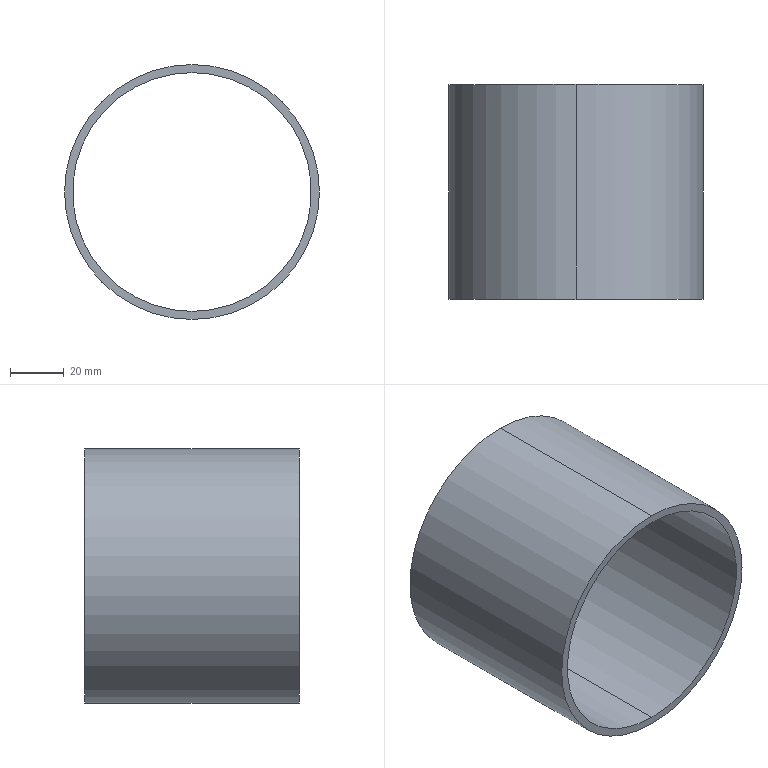Part | SolidWorks | features Extrusion 1 | 1 solid | 6 faces | box 95 x 80 x 95 mm | volume 69366 mm3 | cylinder 4 | plane 2 | commonest cylinder face diameters 89 x2 95 x2
STEP:
#1=CARTESIAN_POINT('',(0.,80.,-44.5));
#2=VERTEX_POINT('',#1);
#3=CARTESIAN_POINT('',(0.,80.,44.5));
#4=VERTEX_POINT('',#3);
#5=CARTESIAN_POINT('',(0.,80.,0.));
#6=DIRECTION('',(0.,1.,0.));
#7=DIRECTION('',(0.,0.,1.));
#8=AXIS2_PLACEMENT_3D('',#5,#6,#7);
#9=CIRCLE('',#8,44.5);
#10=EDGE_CURVE('',#2,#4,#9,.T.);
#11=ORIENTED_EDGE('',*,*,#10,.T.);
#12=CARTESIAN_POINT('',(0.,0.,44.5));
#13=VERTEX_POINT('',#12);
#14=CARTESIAN_POINT('',(0.,80.,44.5));
#15=DIRECTION('',(0.,-1.,0.));
#16=VECTOR('',#15,1000.);
#17=LINE('',#14,#16);
#18=EDGE_CURVE('',#4,#13,#17,.T.);
#19=ORIENTED_EDGE('',*,*,#18,.T.);
#20=CARTESIAN_POINT('',(0.,0.,-44.5));
#21=VERTEX_POINT('',#20);
#22=CARTESIAN_POINT('',(0.,0.,0.));
#23=DIRECTION('',(0.,1.,0.));
#24=DIRECTION('',(0.,0.,1.));
#25=AXIS2_PLACEMENT_3D('',#22,#23,#24);
#26=CIRCLE('',#25,44.5);
#27=EDGE_CURVE('',#21,#13,#26,.T.);
#28=ORIENTED_EDGE('',*,*,#27,.F.);
#29=CARTESIAN_POINT('',(0.,80.,-44.5));
#30=DIRECTION('',(0.,-1.,0.));
#31=VECTOR('',#30,1000.);
#32=LINE('',#29,#31);
#33=EDGE_CURVE('',#2,#21,#32,.T.);
#34=ORIENTED_EDGE('',*,*,#33,.F.);
#35=EDGE_LOOP('',(#11,#19,#28,#34));
#36=FACE_OUTER_BOUND('',#35,.T.);
#37=CARTESIAN_POINT('',(0.,80.,0.));
#38=DIRECTION('',(0.,-1.,0.));
#39=DIRECTION('',(0.,0.,-1.));
#40=AXIS2_PLACEMENT_3D('',#37,#38,#39);
#41=CYLINDRICAL_SURFACE('',#40,44.5);
#42=ADVANCED_FACE('',(#36),#41,.F.);
#43=CARTESIAN_POINT('',(0.,80.,47.5));
#44=VERTEX_POINT('',#43);
#45=CARTESIAN_POINT('',(0.,80.,-47.5));
#46=VERTEX_POINT('',#45);
#47=CARTESIAN_POINT('',(0.,80.,0.));
#48=DIRECTION('',(0.,1.,0.));
#49=DIRECTION('',(0.,0.,1.));
#50=AXIS2_PLACEMENT_3D('',#47,#48,#49);
#51=CIRCLE('',#50,47.5);
#52=EDGE_CURVE('',#44,#46,#51,.T.);
#53=ORIENTED_EDGE('',*,*,#52,.F.);
#54=CARTESIAN_POINT('',(0.,0.,47.5));
#55=VERTEX_POINT('',#54);
#56=CARTESIAN_POINT('',(0.,80.,47.5));
#57=DIRECTION('',(0.,-1.,0.));
#58=VECTOR('',#57,1000.);
#59=LINE('',#56,#58);
#60=EDGE_CURVE('',#44,#55,#59,.T.);
#61=ORIENTED_EDGE('',*,*,#60,.T.);
#62=CARTESIAN_POINT('',(0.,0.,-47.5));
#63=VERTEX_POINT('',#62);
#64=CARTESIAN_POINT('',(0.,0.,0.));
#65=DIRECTION('',(0.,1.,0.));
#66=DIRECTION('',(0.,0.,1.));
#67=AXIS2_PLACEMENT_3D('',#64,#65,#66);
#68=CIRCLE('',#67,47.5);
#69=EDGE_CURVE('',#55,#63,#68,.T.);
#70=ORIENTED_EDGE('',*,*,#69,.T.);
#71=CARTESIAN_POINT('',(0.,80.,-47.5));
#72=DIRECTION('',(0.,-1.,0.));
#73=VECTOR('',#72,1000.);
#74=LINE('',#71,#73);
#75=EDGE_CURVE('',#46,#63,#74,.T.);
#76=ORIENTED_EDGE('',*,*,#75,.F.);
#77=EDGE_LOOP('',(#53,#61,#70,#76));
#78=FACE_OUTER_BOUND('',#77,.T.);
#79=CARTESIAN_POINT('',(0.,80.,0.));
#80=DIRECTION('',(0.,-1.,0.));
#81=DIRECTION('',(0.,0.,-1.));
#82=AXIS2_PLACEMENT_3D('',#79,#80,#81);
#83=CYLINDRICAL_SURFACE('',#82,47.5);
#84=ADVANCED_FACE('',(#78),#83,.T.);
#85=CARTESIAN_POINT('',(0.,80.,0.));
#86=DIRECTION('',(0.,1.,0.));
#87=DIRECTION('',(0.,0.,1.));
#88=AXIS2_PLACEMENT_3D('',#85,#86,#87);
#89=CIRCLE('',#88,47.5);
#90=EDGE_CURVE('',#46,#44,#89,.T.);
#91=ORIENTED_EDGE('',*,*,#90,.T.);
#92=ORIENTED_EDGE('',*,*,#52,.T.);
#93=EDGE_LOOP('',(#91,#92));
#94=FACE_OUTER_BOUND('',#93,.T.);
#95=ORIENTED_EDGE('',*,*,#10,.F.);
#96=CARTESIAN_POINT('',(0.,80.,0.));
#97=DIRECTION('',(0.,1.,0.));
#98=DIRECTION('',(0.,0.,1.));
#99=AXIS2_PLACEMENT_3D('',#96,#97,#98);
#100=CIRCLE('',#99,44.5);
#101=EDGE_CURVE('',#4,#2,#100,.T.);
#102=ORIENTED_EDGE('',*,*,#101,.F.);
#103=EDGE_LOOP('',(#95,#102));
#104=FACE_BOUND('',#103,.T.);
#105=CARTESIAN_POINT('',(0.,80.,0.));
#106=DIRECTION('',(0.,1.,0.));
#107=DIRECTION('',(0.,0.,1.));
#108=AXIS2_PLACEMENT_3D('',#105,#106,#107);
#109=PLANE('',#108);
#110=ADVANCED_FACE('',(#94,#104),#109,.T.);
#111=CARTESIAN_POINT('',(0.,0.,0.));
#112=DIRECTION('',(0.,1.,0.));
#113=DIRECTION('',(0.,0.,1.));
#114=AXIS2_PLACEMENT_3D('',#111,#112,#113);
#115=CIRCLE('',#114,47.5);
#116=EDGE_CURVE('',#63,#55,#115,.T.);
#117=ORIENTED_EDGE('',*,*,#116,.F.);
#118=ORIENTED_EDGE('',*,*,#69,.F.);
#119=EDGE_LOOP('',(#117,#118));
#120=FACE_OUTER_BOUND('',#119,.T.);
#121=ORIENTED_EDGE('',*,*,#27,.T.);
#122=CARTESIAN_POINT('',(0.,0.,0.));
#123=DIRECTION('',(0.,1.,0.));
#124=DIRECTION('',(0.,0.,1.));
#125=AXIS2_PLACEMENT_3D('',#122,#123,#124);
#126=CIRCLE('',#125,44.5);
#127=EDGE_CURVE('',#13,#21,#126,.T.);
#128=ORIENTED_EDGE('',*,*,#127,.T.);
#129=EDGE_LOOP('',(#121,#128));
#130=FACE_BOUND('',#129,.T.);
#131=CARTESIAN_POINT('',(0.,0.,0.));
#132=DIRECTION('',(0.,1.,0.));
#133=DIRECTION('',(0.,0.,1.));
#134=AXIS2_PLACEMENT_3D('',#131,#132,#133);
#135=PLANE('',#134);
#136=ADVANCED_FACE('',(#120,#130),#135,.F.);
#137=ORIENTED_EDGE('',*,*,#60,.F.);
#138=ORIENTED_EDGE('',*,*,#90,.F.);
#139=ORIENTED_EDGE('',*,*,#75,.T.);
#140=ORIENTED_EDGE('',*,*,#116,.T.);
#141=EDGE_LOOP('',(#137,#138,#139,#140));
#142=FACE_OUTER_BOUND('',#141,.T.);
#143=CARTESIAN_POINT('',(0.,80.,0.));
#144=DIRECTION('',(0.,-1.,0.));
#145=DIRECTION('',(0.,0.,-1.));
#146=AXIS2_PLACEMENT_3D('',#143,#144,#145);
#147=CYLINDRICAL_SURFACE('',#146,47.5);
#148=ADVANCED_FACE('',(#142),#147,.T.);
#149=ORIENTED_EDGE('',*,*,#18,.F.);
#150=ORIENTED_EDGE('',*,*,#101,.T.);
#151=ORIENTED_EDGE('',*,*,#33,.T.);
#152=ORIENTED_EDGE('',*,*,#127,.F.);
#153=EDGE_LOOP('',(#149,#150,#151,#152));
#154=FACE_OUTER_BOUND('',#153,.T.);
#155=CARTESIAN_POINT('',(0.,80.,0.));
#156=DIRECTION('',(0.,-1.,0.));
#157=DIRECTION('',(0.,0.,-1.));
#158=AXIS2_PLACEMENT_3D('',#155,#156,#157);
#159=CYLINDRICAL_SURFACE('',#158,44.5);
#160=ADVANCED_FACE('',(#154),#159,.F.);
#161=CLOSED_SHELL('',(#42,#84,#110,#136,#148,#160));
#162=MANIFOLD_SOLID_BREP('',#161);
#163=CARTESIAN_POINT('',(0.,0.,0.));
#164=DIRECTION('',(0.,0.,1.));
#165=DIRECTION('',(1.,0.,0.));
#166=AXIS2_PLACEMENT_3D('',#163,#164,#165);
#167=(LENGTH_UNIT()NAMED_UNIT(*)SI_UNIT(.MILLI.,.METRE.));
#168=UNCERTAINTY_MEASURE_WITH_UNIT(LENGTH_MEASURE(0.00001),#167,'','');
#169=(NAMED_UNIT(*)PLANE_ANGLE_UNIT()SI_UNIT($,.RADIAN.));
#170=(NAMED_UNIT(*)SI_UNIT($,.STERADIAN.)SOLID_ANGLE_UNIT());
#171=(GEOMETRIC_REPRESENTATION_CONTEXT(3)GLOBAL_UNCERTAINTY_ASSIGNED_CONTEXT((#168))GLOBAL_UNIT_ASSIGNED_CONTEXT((#167,#169,#170))REPRESENTATION_CONTEXT('',''));
#172=ADVANCED_BREP_SHAPE_REPRESENTATION('',(#162,#166),#171);